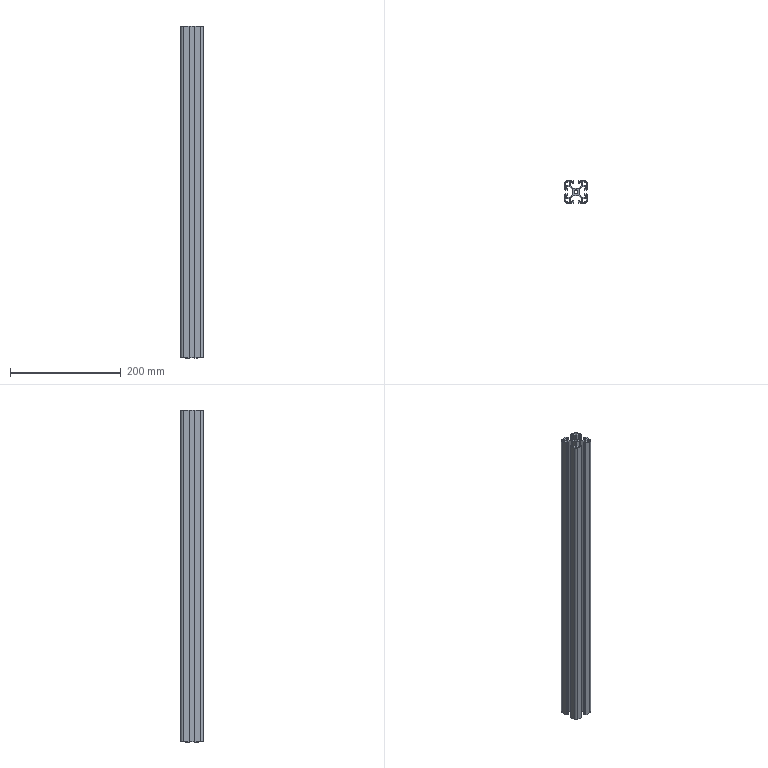Part | STEP file | LE-8-4040-S-OO_LE0314200037 | 1 solid | 188 faces | box 40 x 40 x 600 mm | volume 286949 mm3 | cylinder 94 | plane 94 | commonest cylinder face diameters 0.6 x30 2 x28 4 x16 0.4 x8 6 x4 9 x4